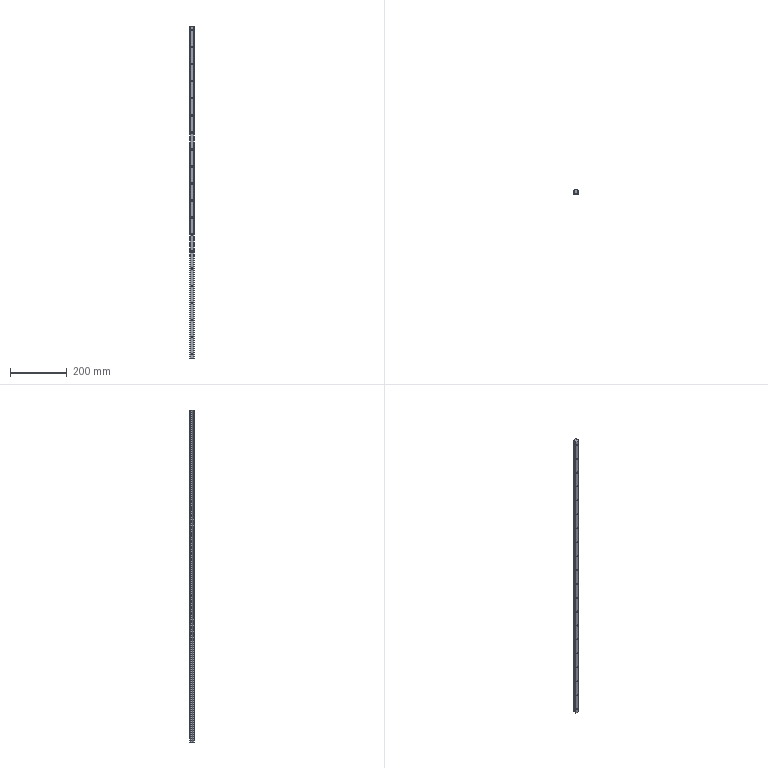Part | STEP file | HGR15-1170 | 1 solid | 136 faces | box 15 x 15 x 1170 mm | volume 215420 mm3 | cylinder 94 | plane 42 | commonest cylinder face diameters 4.5 x40 7.5 x40 0.8 x8 3.24 x4 2 x2